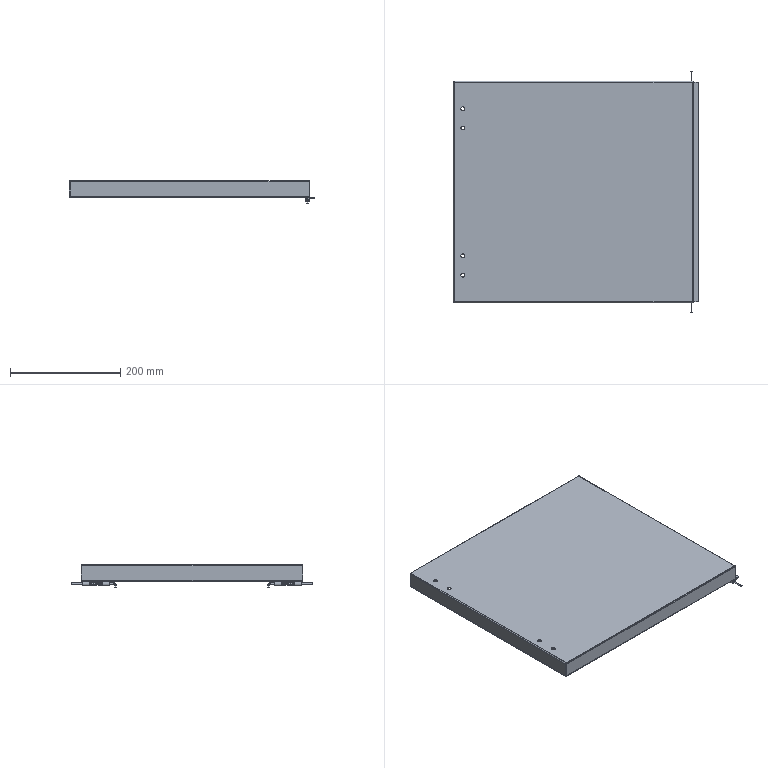Part | 5 solids | 145 faces | box 444.8 x 438.127 x 41 mm | volume 290283 mm3 | plane 76 | cylinder 51 | spline 14 | torus 4 | commonest cylinder face diameters 7 x11 1.473 x8 3 x8 3.6 x8 3.873 x8 7.6 x8